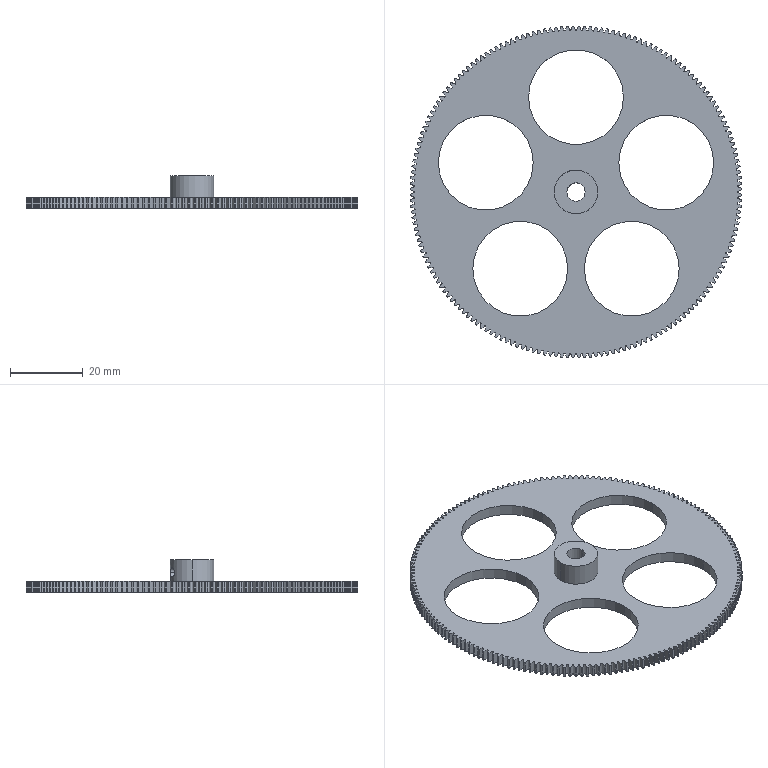Part | SolidWorks | features ICE 3, 3DProfileFeature 1, CirPattern 1, HoleWzd 1, RefAxis 1, Revolution 1 | 1 solid | 379 faces | box 90.992 x 90.992 x 9 mm | volume 9929 mm3 | cylinder 196 | spline 180 | plane 3 | commonest cylinder face diameters 91 x180 26 x10 2.5 x2 5 x2 12 x2